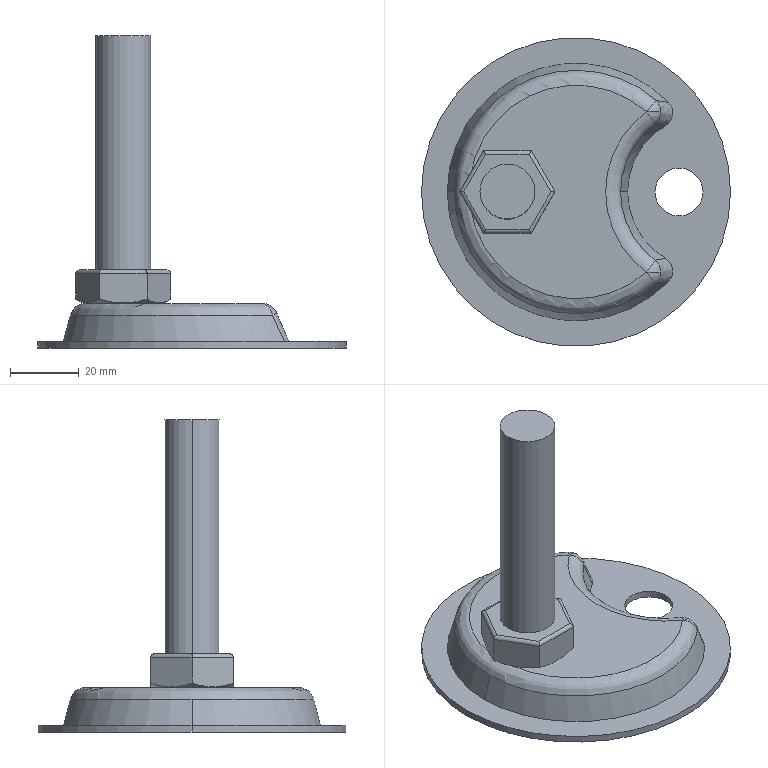Part | SolidWorks | features BaseBody 1 | 1 solid | 81 faces | box 90 x 90 x 91 mm | volume 39488 mm3 | plane 27 | cone 20 | cylinder 16 | sphere 8 | torus 6 | spline 4 | commonest cylinder face diameters 2 x6 16 x4 14 x2 17 x2 90 x2